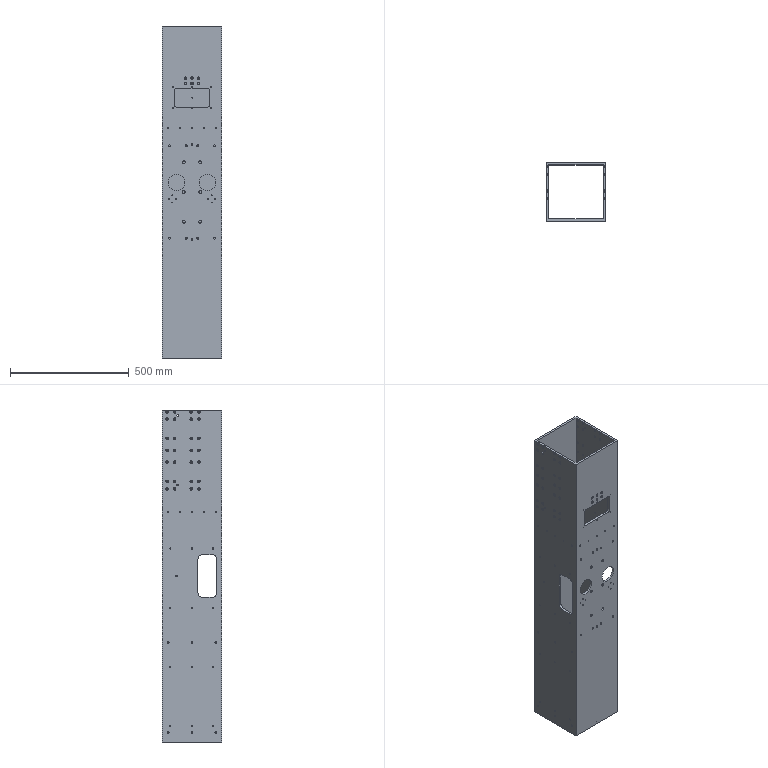Part | SolidWorks | features HoleWzd 16, Cut 2, Fillet 2, ICE 2, Extrusion 1 | 1 solid | 571 faces | box 250 x 250 x 1400 mm | volume 12885906 mm3 | cylinder 469 | plane 86 | cone 16 | commonest cylinder face diameters 7 x124 11 x124 5 x88 3.3 x30 6.8 x28 4.2 x16